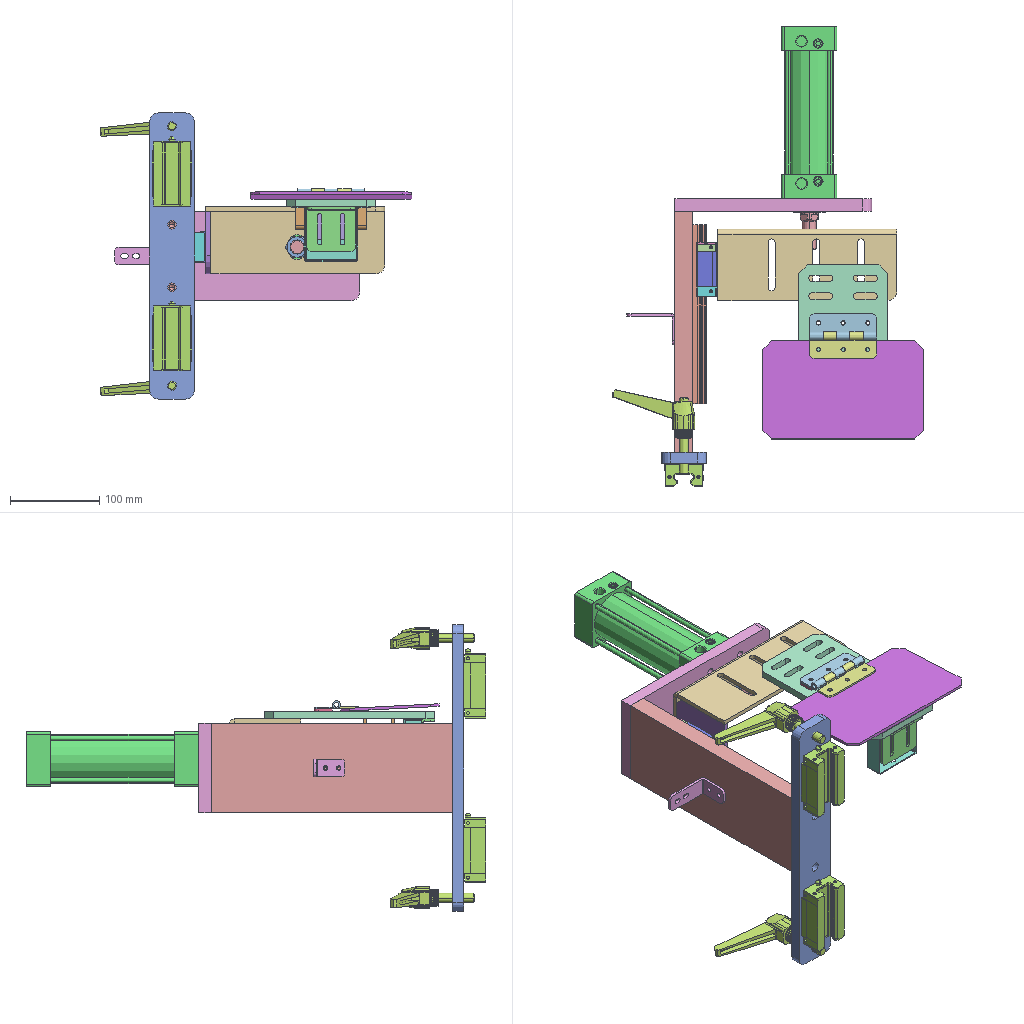Assembly | SolidWorks | 23 different items | 25 placed | box 348 x 514 x 320 mm
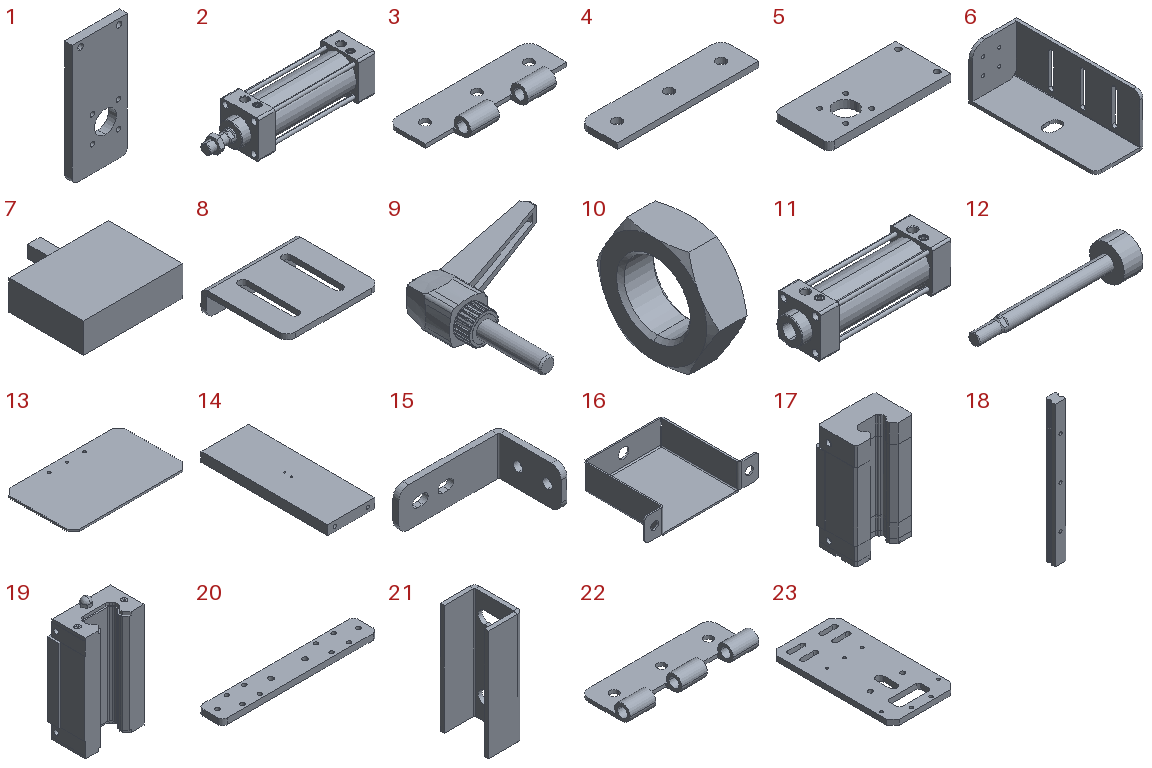Parts list (item | name | quantity | parent item | size | volume | features):
1 | (subassembly) | x1 | - | 100 x 14 x 220 mm | 284792 mm3 | features CompositeCurve 43
2 | (subassembly) | x1 | - | 250 x 62 x 62 mm | 379695 mm3 | -
3 | - | x1 | - | 75 x 29.3 x 9.25 mm | 4196 mm3 | features Extrusion 1, Fillet 1, ICE 1, LPattern 1
4 | - | x1 | - | 75 x 20 x 3 mm | 4291 mm3 | features Extrusion 1, Fillet 1
5 | - | x1 | in 1 | 220 x 100 x 14 mm | 284792 mm3 | features Fillet 1, FlatPattern 1, SMBaseFlange 1, SheetMetal 1
6 | - | x1 | - | 75 x 200 x 80 mm | 164738 mm3 | features ICE 4, Fillet 2, EdgeFlange 1, FlatPattern 1, SMBaseFlange 1, SheetMetal 1
7 | - | x1 | - | 40 x 40 x 12 mm | 14775 mm3 | features Extrusion 1, ICE 1
8 | - | x1 | - | 54 x 50 x 15 mm | 8636 mm3 | features EdgeFlange 1, Extrusion 1, Fillet 1, FlatPattern 1, ICE 1, SheetMetal 1, SolidToSheetMetal 1
9 | - | x2 | - | 92 x 94 x 24 mm | 28116 mm3 | features ICE 2, BaseBody 1, Chamfer 1
10 | - | x1 | in 2 | 8 x 26.558 x 23 mm | 2309 mm3 | features BaseBody 1
11 | - | x1 | in 2 | 208 x 62 x 62 mm | 269760 mm3 | features BaseBody 1
12 | - | x1 | in 2 | 217 x 49.5 x 49.5 mm | 107628 mm3 | features BaseBody 1
13 | - | x1 | - | 180 x 110 x 3 mm | 58687 mm3 | features Extrusion 1
14 | - | x1 | - | 100 x 270 x 20 mm | 536586 mm3 | features HoleWzd 3, 3DProfileFeature 1, Extrusion 1
15 | - | x1 | - | 54 x 35 x 20 mm | 4722 mm3 | features Fillet 1, FlatPattern 1, HoleWzd 1, ICE 1, SMBaseFlange 1, SheetMetal 1
16 | - | x1 | - | 87.6 x 61.2 x 20 mm | 8600 mm3 | features EdgeFlange 2, Fillet 1, FlatPattern 1, ICE 1, SMBaseFlange 1, SheetMetal 1
17 | - | x1 | - | 34.1 x 23.6 x 60.875 mm | 38055 mm3 | features ICE 19, MirrorPattern 4, Chamfer 3, Extrusion 3, MirrorSolid 3, Fillet 2, Dome 1, RevCut 1, Revolution 1
18 | - | x1 | - | 15 x 15 x 200 mm | 39273 mm3 | features ICE 15, Chamfer 3, Extrusion 3, Fillet 3, MirrorPattern 3, MirrorSolid 3, RevCut 2, DeleteBody 1, Dome 1, LPattern 1
19 | - | x2 | - | 44 x 25 x 77.9 mm | 57159 mm3 | features ICE 10, MirrorPattern 3, Chamfer 1, Extrusion 1, HoleWzd 1, Revolution 1
20 | - | x1 | - | 320 x 50 x 12 mm | 182898 mm3 | features Extrusion 1, Fillet 1, HoleWzd 1
21 | - | x1 | - | 25 x 35 x 80 mm | 16996 mm3 | features EdgeFlange 1, FlatPattern 1, SMBaseFlange 1, SheetMetal 1
22 | - | x1 | - | 75 x 29.3 x 9.25 mm | 4864 mm3 | features Extrusion 1, Fillet 1, ICE 1, LPattern 1
23 | - | x1 | - | 100 x 190 x 8 mm | 132589 mm3 | features 3DProfileFeature 2, HoleWzd 2, Chamfer 1, Extrusion 1, ICE 1, LPattern 1
Mates (type | each side: item.copy, entity, surface, feature):
In the top assembly
Coincident | 14.1 face plane Boss-Extrude1 | 20.1 face plane Boss-Extrude1
Concentric | 20.1 face cylinder Boss-Extrude1 | 14.1 face cylinder M8 Tapped Hole1 | 2 times
Coincident | 5.1 face plane Base-Flange1 | 14.1 face plane Boss-Extrude1 | 3 times
Coincident | 18.1 face plane Boss-Extrude8 | 14.1 face plane Boss-Extrude1
Coincident | 19.1 face plane Boss-Extrude1 | 20.1 face plane Boss-Extrude1
Concentric | 19.2 face cylinder threaded hole 1 | 20.1 face cylinder Boss-Extrude1 | 2 times
Coincident | 19.2 face plane Boss-Extrude1 | 20.1 face plane Boss-Extrude1
Coincident | assembly face | 6.1 face plane Base-Flange1
Width | 23.1 face plane Boss-Extrude1 | 23.1 face plane Boss-Extrude1 | assembly face | assembly face | 2 times
Coincident | 23.1 face plane Boss-Extrude1 | 6.1 face plane Edge-Flange1
Parallel | 23.1 edge | 6.1 face plane Base-Flange1
Coincident | 4.1 face plane Boss-Extrude1 | 22.1 face plane Boss-Extrude1
Coincident | 4.1 face cylinder Boss-Extrude1 | 22.1 edge | 2 times
Concentric | 22.1 face cylinder Boss-Extrude2 | 3.1 face cylinder LPattern1
Coincident | 22.1 face plane LPattern1 | 3.1 face plane LPattern1
Coincident | 3.1 face plane Boss-Extrude1 | 13.1 face plane Boss-Extrude1
Concentric | 3.1 edge | 13.1 edge | 2 times
Coincident | 23.1 face plane Boss-Extrude1 | 4.1 face plane Boss-Extrude1
Concentric | 23.1 edge | 4.1 edge
Concentric | 23.1 face cylinder Boss-Extrude1 | 22.1 face cylinder Boss-Extrude1
Coincident | 8.1 face plane Convert Entities1 | 7.1 face plane Boss-Extrude1
Width | 8.1 face plane Convert Entities1 | 8.1 face plane Convert Entities1 | 7.1 face plane Boss-Extrude1 | 7.1 face plane Boss-Extrude1
DistanceDim | 7.1 face plane Boss-Extrude1 | 8.1 face plane Convert Entities1
Coincident | 23.1 face plane Boss-Extrude1 | 16.1 face plane Edge-Flange2
Width | 23.1 face plane Boss-Extrude1 | 23.1 face plane Boss-Extrude1 | 16.1 face plane Edge-Flange1 | 16.1 face plane Edge-Flange1
DistanceDim | 23.1 face plane Boss-Extrude1 | 16.1 face plane Edge-Flange1
Coincident | 23.1 face plane Boss-Extrude1 | 21.1 face plane Edge-Flange1
Width | 23.1 face plane Boss-Extrude1 | 23.1 face plane Boss-Extrude1 | 21.1 face plane Edge-Flange1 | 21.1 face plane Edge-Flange1
DistanceDim | 21.1 face plane Edge-Flange1 | 23.1 face plane Boss-Extrude1
Coincident | 23.1 face plane Boss-Extrude1 | 8.1 face plane Edge-Flange2
Concentric | 23.1 face cylinder Boss-Extrude1 | 8.1 face cylinder Cut-Extrude1 | 2 times
DistanceDim | 20.1 face plane Boss-Extrude1 | 18.1 face plane Boss-Extrude8
Concentric | 19.1 face cylinder threaded hole 1 | 20.1 face cylinder Boss-Extrude1 | 2 times
Concentric | 5.1 face cylinder Base-Flange1 | 11.1 face cylinder Input1 | 2 times
Coincident | 5.1 face plane Base-Flange1 | 11.1 face plane Input1
Width | 17.1 face plane Boss-Extrude1 | 17.1 face plane Boss-Extrude1 | 18.1 face cylinder LPattern1
DistanceDim | 17.1 face plane Boss-Extrude1 | 14.1 face plane Boss-Extrude1
Coincident | 17.1 face plane Boss-Extrude1 | 6.1 face plane Boss-Extrude1
Parallel | 5.1 face plane Base-Flange1 | 6.1 face plane Base-Flange1
LimitDistanceDim | 5.1 face plane Base-Flange1 | 6.1 face plane Base-Flange1
Concentric | 17.1 edge | 6.1 face cylinder Cut-Extrude4
Concentric | 17.1 face cylinder Cut-Revolve1 | 6.1 face cylinder Cut-Extrude4
DistanceDim | 23.1 edge | 6.1 face plane Boss-Extrude1
DistanceDim | 23.1 face plane Boss-Extrude1 | 6.1 face plane Base-Flange1
DistanceDim | 18.1 face plane Boss-Extrude8 | 14.1 face plane Boss-Extrude1
Concentric | 20.1 face cylinder M10 Tapped Hole1 | 9.1 face cylinder Cut-Extrude2
Coincident | 19.2 face plane Cut-Extrude2 | 9.1 face plane Cut-Extrude1
Concentric | 20.1 face cylinder M10 Tapped Hole1 | 9.2 face cylinder Cut-Extrude2
Coincident | 9.1 face plane Cut-Extrude1 | 9.2 face plane Cut-Extrude1
Coincident | 14.1 face plane Boss-Extrude1 | 15.1 face plane Base-Flange1
Concentric | 14.1 face cylinder M4 Tapped Hole2 | 15.1 edge
In subassembly 2
LimitDistanceDim | 12.1 face plane Input1 | 11.2 face plane Input1
DistanceDim | 12.1 face plane Input1 | 10.1 face plane Input1